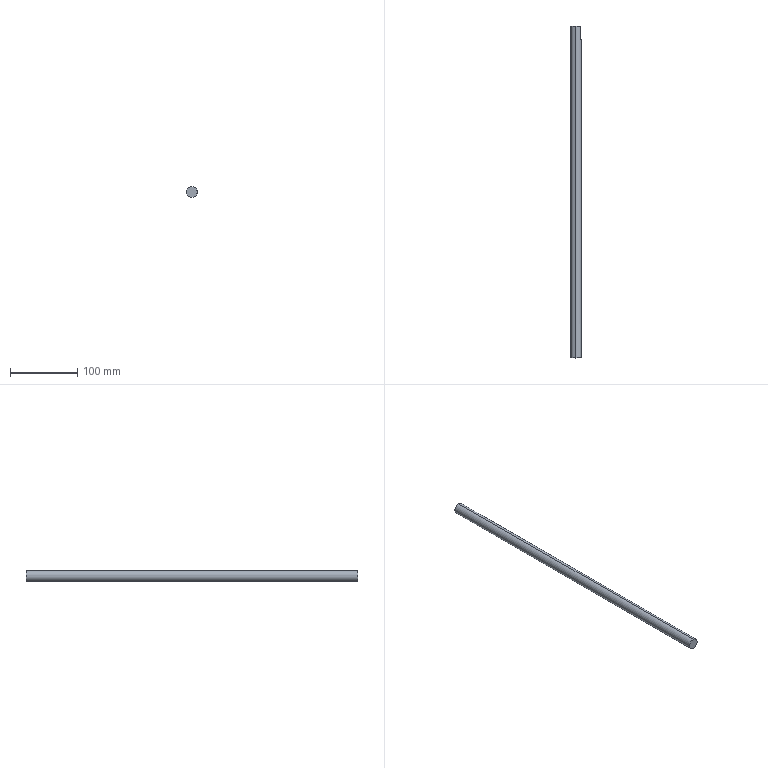Part | SolidWorks | features Extrusion 1, ICE 1 | 1 solid | 6 faces | box 16 x 495 x 16 mm | volume 99236 mm3 | plane 4 | cylinder 2 | commonest cylinder face diameters 16 x2
STEP:
#1=CARTESIAN_POINT('',(0.,495.,8.));
#2=VERTEX_POINT('',#1);
#3=CARTESIAN_POINT('',(6.,495.,5.292));
#4=VERTEX_POINT('',#3);
#5=CARTESIAN_POINT('',(0.,495.,0.));
#6=DIRECTION('',(0.,1.,0.));
#7=DIRECTION('',(0.,0.,1.));
#8=AXIS2_PLACEMENT_3D('',#5,#6,#7);
#9=CIRCLE('',#8,8.);
#10=EDGE_CURVE('',#2,#4,#9,.T.);
#11=ORIENTED_EDGE('',*,*,#10,.F.);
#12=CARTESIAN_POINT('',(0.,0.,8.));
#13=VERTEX_POINT('',#12);
#14=CARTESIAN_POINT('',(0.,495.,8.));
#15=DIRECTION('',(0.,-1.,0.));
#16=VECTOR('',#15,1000.);
#17=LINE('',#14,#16);
#18=EDGE_CURVE('',#2,#13,#17,.T.);
#19=ORIENTED_EDGE('',*,*,#18,.T.);
#20=CARTESIAN_POINT('',(0.,0.,-8.));
#21=VERTEX_POINT('',#20);
#22=CARTESIAN_POINT('',(0.,0.,0.));
#23=DIRECTION('',(0.,1.,0.));
#24=DIRECTION('',(0.,0.,1.));
#25=AXIS2_PLACEMENT_3D('',#22,#23,#24);
#26=CIRCLE('',#25,8.);
#27=EDGE_CURVE('',#13,#21,#26,.T.);
#28=ORIENTED_EDGE('',*,*,#27,.T.);
#29=CARTESIAN_POINT('',(0.,495.,-8.));
#30=VERTEX_POINT('',#29);
#31=CARTESIAN_POINT('',(0.,495.,-8.));
#32=DIRECTION('',(0.,-1.,0.));
#33=VECTOR('',#32,1000.);
#34=LINE('',#31,#33);
#35=EDGE_CURVE('',#30,#21,#34,.T.);
#36=ORIENTED_EDGE('',*,*,#35,.F.);
#37=CARTESIAN_POINT('',(6.,495.,-5.292));
#38=VERTEX_POINT('',#37);
#39=CARTESIAN_POINT('',(0.,495.,0.));
#40=DIRECTION('',(0.,1.,0.));
#41=DIRECTION('',(0.,0.,1.));
#42=AXIS2_PLACEMENT_3D('',#39,#40,#41);
#43=CIRCLE('',#42,8.);
#44=EDGE_CURVE('',#38,#30,#43,.T.);
#45=ORIENTED_EDGE('',*,*,#44,.F.);
#46=CARTESIAN_POINT('',(6.,475.,-5.292));
#47=VERTEX_POINT('',#46);
#48=CARTESIAN_POINT('',(6.,495.,-5.292));
#49=DIRECTION('',(0.,-1.,0.));
#50=VECTOR('',#49,1000.);
#51=LINE('',#48,#50);
#52=EDGE_CURVE('',#38,#47,#51,.T.);
#53=ORIENTED_EDGE('',*,*,#52,.T.);
#54=CARTESIAN_POINT('',(6.,475.,5.292));
#55=VERTEX_POINT('',#54);
#56=CARTESIAN_POINT('',(0.,475.,0.));
#57=DIRECTION('',(0.,-1.,0.));
#58=DIRECTION('',(0.,0.,-1.));
#59=AXIS2_PLACEMENT_3D('',#56,#57,#58);
#60=CIRCLE('',#59,8.);
#61=EDGE_CURVE('',#47,#55,#60,.T.);
#62=ORIENTED_EDGE('',*,*,#61,.T.);
#63=CARTESIAN_POINT('',(6.,495.,5.292));
#64=DIRECTION('',(0.,1.,0.));
#65=VECTOR('',#64,1000.);
#66=LINE('',#63,#65);
#67=EDGE_CURVE('',#55,#4,#66,.T.);
#68=ORIENTED_EDGE('',*,*,#67,.T.);
#69=EDGE_LOOP('',(#11,#19,#28,#36,#45,#53,#62,#68));
#70=FACE_OUTER_BOUND('',#69,.T.);
#71=CARTESIAN_POINT('',(0.,495.,0.));
#72=DIRECTION('',(0.,-1.,0.));
#73=DIRECTION('',(0.,0.,-1.));
#74=AXIS2_PLACEMENT_3D('',#71,#72,#73);
#75=CYLINDRICAL_SURFACE('',#74,8.);
#76=ADVANCED_FACE('',(#70),#75,.T.);
#77=ORIENTED_EDGE('',*,*,#18,.F.);
#78=CARTESIAN_POINT('',(0.,495.,0.));
#79=DIRECTION('',(0.,1.,0.));
#80=DIRECTION('',(0.,0.,1.));
#81=AXIS2_PLACEMENT_3D('',#78,#79,#80);
#82=CIRCLE('',#81,8.);
#83=EDGE_CURVE('',#30,#2,#82,.T.);
#84=ORIENTED_EDGE('',*,*,#83,.F.);
#85=ORIENTED_EDGE('',*,*,#35,.T.);
#86=CARTESIAN_POINT('',(0.,0.,0.));
#87=DIRECTION('',(0.,1.,0.));
#88=DIRECTION('',(0.,0.,1.));
#89=AXIS2_PLACEMENT_3D('',#86,#87,#88);
#90=CIRCLE('',#89,8.);
#91=EDGE_CURVE('',#21,#13,#90,.T.);
#92=ORIENTED_EDGE('',*,*,#91,.T.);
#93=EDGE_LOOP('',(#77,#84,#85,#92));
#94=FACE_OUTER_BOUND('',#93,.T.);
#95=CARTESIAN_POINT('',(0.,495.,0.));
#96=DIRECTION('',(0.,-1.,0.));
#97=DIRECTION('',(0.,0.,-1.));
#98=AXIS2_PLACEMENT_3D('',#95,#96,#97);
#99=CYLINDRICAL_SURFACE('',#98,8.);
#100=ADVANCED_FACE('',(#94),#99,.T.);
#101=CARTESIAN_POINT('',(6.,495.,0.));
#102=DIRECTION('',(0.,0.,1.));
#103=VECTOR('',#102,1000.);
#104=LINE('',#101,#103);
#105=EDGE_CURVE('',#38,#4,#104,.T.);
#106=ORIENTED_EDGE('',*,*,#105,.F.);
#107=ORIENTED_EDGE('',*,*,#44,.T.);
#108=ORIENTED_EDGE('',*,*,#83,.T.);
#109=ORIENTED_EDGE('',*,*,#10,.T.);
#110=EDGE_LOOP('',(#106,#107,#108,#109));
#111=FACE_OUTER_BOUND('',#110,.T.);
#112=CARTESIAN_POINT('',(0.,495.,0.));
#113=DIRECTION('',(0.,1.,0.));
#114=DIRECTION('',(0.,0.,1.));
#115=AXIS2_PLACEMENT_3D('',#112,#113,#114);
#116=PLANE('',#115);
#117=ADVANCED_FACE('',(#111),#116,.T.);
#118=ORIENTED_EDGE('',*,*,#91,.F.);
#119=ORIENTED_EDGE('',*,*,#27,.F.);
#120=EDGE_LOOP('',(#118,#119));
#121=FACE_OUTER_BOUND('',#120,.T.);
#122=CARTESIAN_POINT('',(0.,0.,0.));
#123=DIRECTION('',(0.,1.,0.));
#124=DIRECTION('',(0.,0.,1.));
#125=AXIS2_PLACEMENT_3D('',#122,#123,#124);
#126=PLANE('',#125);
#127=ADVANCED_FACE('',(#121),#126,.F.);
#128=CARTESIAN_POINT('',(6.,475.,-8.));
#129=DIRECTION('',(0.,0.,1.));
#130=VECTOR('',#129,1000.);
#131=LINE('',#128,#130);
#132=EDGE_CURVE('',#47,#55,#131,.T.);
#133=ORIENTED_EDGE('',*,*,#132,.T.);
#134=ORIENTED_EDGE('',*,*,#61,.F.);
#135=EDGE_LOOP('',(#133,#134));
#136=FACE_OUTER_BOUND('',#135,.T.);
#137=CARTESIAN_POINT('',(8.,475.,-8.));
#138=DIRECTION('',(0.,-1.,0.));
#139=DIRECTION('',(0.,0.,-1.));
#140=AXIS2_PLACEMENT_3D('',#137,#138,#139);
#141=PLANE('',#140);
#142=ADVANCED_FACE('',(#136),#141,.F.);
#143=ORIENTED_EDGE('',*,*,#105,.T.);
#144=ORIENTED_EDGE('',*,*,#67,.F.);
#145=ORIENTED_EDGE('',*,*,#132,.F.);
#146=ORIENTED_EDGE('',*,*,#52,.F.);
#147=EDGE_LOOP('',(#143,#144,#145,#146));
#148=FACE_OUTER_BOUND('',#147,.T.);
#149=CARTESIAN_POINT('',(6.,475.,-8.));
#150=DIRECTION('',(-1.,0.,0.));
#151=DIRECTION('',(0.,0.,1.));
#152=AXIS2_PLACEMENT_3D('',#149,#150,#151);
#153=PLANE('',#152);
#154=ADVANCED_FACE('',(#148),#153,.F.);
#155=CLOSED_SHELL('',(#76,#100,#117,#127,#142,#154));
#156=MANIFOLD_SOLID_BREP('',#155);
#157=CARTESIAN_POINT('',(0.,0.,0.));
#158=DIRECTION('',(0.,0.,1.));
#159=DIRECTION('',(1.,0.,0.));
#160=AXIS2_PLACEMENT_3D('',#157,#158,#159);
#161=(LENGTH_UNIT()NAMED_UNIT(*)SI_UNIT(.MILLI.,.METRE.));
#162=UNCERTAINTY_MEASURE_WITH_UNIT(LENGTH_MEASURE(0.00001),#161,'','');
#163=(NAMED_UNIT(*)PLANE_ANGLE_UNIT()SI_UNIT($,.RADIAN.));
#164=(NAMED_UNIT(*)SI_UNIT($,.STERADIAN.)SOLID_ANGLE_UNIT());
#165=(GEOMETRIC_REPRESENTATION_CONTEXT(3)GLOBAL_UNCERTAINTY_ASSIGNED_CONTEXT((#162))GLOBAL_UNIT_ASSIGNED_CONTEXT((#161,#163,#164))REPRESENTATION_CONTEXT('',''));
#166=ADVANCED_BREP_SHAPE_REPRESENTATION('',(#156,#160),#165);